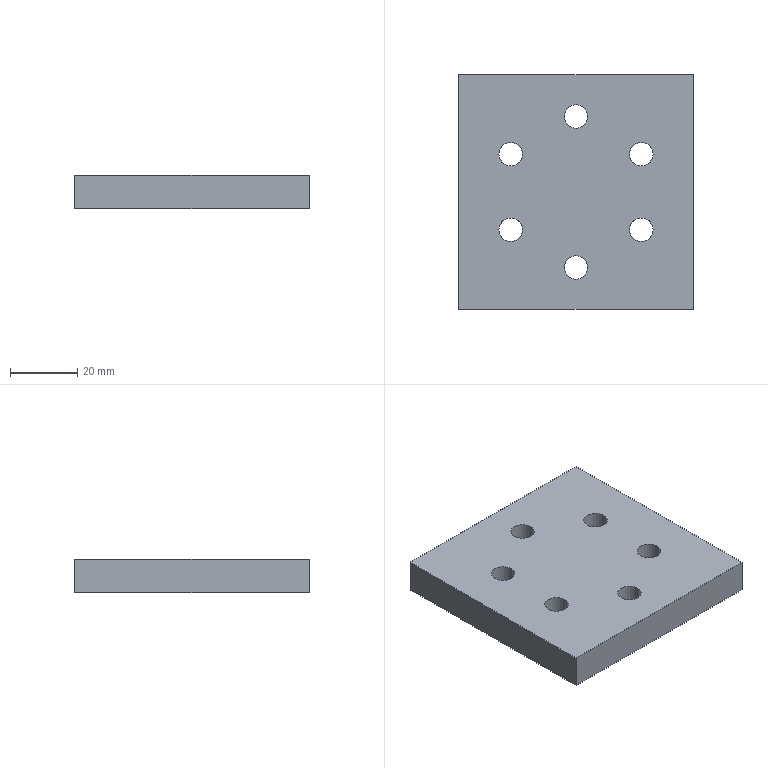Part | SolidWorks | features BaseBody 1 | 1 solid | 18 faces | box 70 x 70 x 10 mm | volume 46691 mm3 | cylinder 12 | plane 6 | commonest cylinder face diameters 7 x12
STEP:
#1=CARTESIAN_POINT('',(15.986,-11.25,0.));
#2=VERTEX_POINT('',#1);
#3=CARTESIAN_POINT('',(22.986,-11.25,0.));
#4=VERTEX_POINT('',#3);
#5=CARTESIAN_POINT('',(19.486,-11.25,0.));
#6=DIRECTION('',(0.,0.,1.));
#7=DIRECTION('',(1.,0.,0.));
#8=AXIS2_PLACEMENT_3D('',#5,#6,#7);
#9=CIRCLE('',#8,3.5);
#10=EDGE_CURVE('',#2,#4,#9,.T.);
#11=ORIENTED_EDGE('',*,*,#10,.F.);
#12=CARTESIAN_POINT('',(15.986,-11.25,10.));
#13=VERTEX_POINT('',#12);
#14=CARTESIAN_POINT('',(15.986,-11.25,10.));
#15=DIRECTION('',(0.,0.,1.));
#16=VECTOR('',#15,1000.);
#17=LINE('',#14,#16);
#18=EDGE_CURVE('',#2,#13,#17,.T.);
#19=ORIENTED_EDGE('',*,*,#18,.T.);
#20=CARTESIAN_POINT('',(22.986,-11.25,10.));
#21=VERTEX_POINT('',#20);
#22=CARTESIAN_POINT('',(19.486,-11.25,10.));
#23=DIRECTION('',(0.,0.,1.));
#24=DIRECTION('',(1.,0.,0.));
#25=AXIS2_PLACEMENT_3D('',#22,#23,#24);
#26=CIRCLE('',#25,3.5);
#27=EDGE_CURVE('',#13,#21,#26,.T.);
#28=ORIENTED_EDGE('',*,*,#27,.T.);
#29=CARTESIAN_POINT('',(22.986,-11.25,10.));
#30=DIRECTION('',(0.,0.,1.));
#31=VECTOR('',#30,1000.);
#32=LINE('',#29,#31);
#33=EDGE_CURVE('',#4,#21,#32,.T.);
#34=ORIENTED_EDGE('',*,*,#33,.F.);
#35=EDGE_LOOP('',(#11,#19,#28,#34));
#36=FACE_OUTER_BOUND('',#35,.T.);
#37=CARTESIAN_POINT('',(19.486,-11.25,10.));
#38=DIRECTION('',(0.,0.,1.));
#39=DIRECTION('',(1.,0.,0.));
#40=AXIS2_PLACEMENT_3D('',#37,#38,#39);
#41=CYLINDRICAL_SURFACE('',#40,3.5);
#42=ADVANCED_FACE('',(#36),#41,.F.);
#43=CARTESIAN_POINT('',(-3.5,-22.5,0.));
#44=VERTEX_POINT('',#43);
#45=CARTESIAN_POINT('',(3.5,-22.5,0.));
#46=VERTEX_POINT('',#45);
#47=CARTESIAN_POINT('',(0.,-22.5,0.));
#48=DIRECTION('',(0.,0.,1.));
#49=DIRECTION('',(1.,0.,0.));
#50=AXIS2_PLACEMENT_3D('',#47,#48,#49);
#51=CIRCLE('',#50,3.5);
#52=EDGE_CURVE('',#44,#46,#51,.T.);
#53=ORIENTED_EDGE('',*,*,#52,.F.);
#54=CARTESIAN_POINT('',(-3.5,-22.5,10.));
#55=VERTEX_POINT('',#54);
#56=CARTESIAN_POINT('',(-3.5,-22.5,10.));
#57=DIRECTION('',(0.,0.,1.));
#58=VECTOR('',#57,1000.);
#59=LINE('',#56,#58);
#60=EDGE_CURVE('',#44,#55,#59,.T.);
#61=ORIENTED_EDGE('',*,*,#60,.T.);
#62=CARTESIAN_POINT('',(3.5,-22.5,10.));
#63=VERTEX_POINT('',#62);
#64=CARTESIAN_POINT('',(0.,-22.5,10.));
#65=DIRECTION('',(0.,0.,1.));
#66=DIRECTION('',(1.,0.,0.));
#67=AXIS2_PLACEMENT_3D('',#64,#65,#66);
#68=CIRCLE('',#67,3.5);
#69=EDGE_CURVE('',#55,#63,#68,.T.);
#70=ORIENTED_EDGE('',*,*,#69,.T.);
#71=CARTESIAN_POINT('',(3.5,-22.5,10.));
#72=DIRECTION('',(0.,0.,1.));
#73=VECTOR('',#72,1000.);
#74=LINE('',#71,#73);
#75=EDGE_CURVE('',#46,#63,#74,.T.);
#76=ORIENTED_EDGE('',*,*,#75,.F.);
#77=EDGE_LOOP('',(#53,#61,#70,#76));
#78=FACE_OUTER_BOUND('',#77,.T.);
#79=CARTESIAN_POINT('',(0.,-22.5,10.));
#80=DIRECTION('',(0.,0.,1.));
#81=DIRECTION('',(1.,0.,0.));
#82=AXIS2_PLACEMENT_3D('',#79,#80,#81);
#83=CYLINDRICAL_SURFACE('',#82,3.5);
#84=ADVANCED_FACE('',(#78),#83,.F.);
#85=CARTESIAN_POINT('',(-22.986,-11.25,0.));
#86=VERTEX_POINT('',#85);
#87=CARTESIAN_POINT('',(-15.986,-11.25,0.));
#88=VERTEX_POINT('',#87);
#89=CARTESIAN_POINT('',(-19.486,-11.25,0.));
#90=DIRECTION('',(0.,0.,1.));
#91=DIRECTION('',(1.,0.,0.));
#92=AXIS2_PLACEMENT_3D('',#89,#90,#91);
#93=CIRCLE('',#92,3.5);
#94=EDGE_CURVE('',#86,#88,#93,.T.);
#95=ORIENTED_EDGE('',*,*,#94,.F.);
#96=CARTESIAN_POINT('',(-22.986,-11.25,10.));
#97=VERTEX_POINT('',#96);
#98=CARTESIAN_POINT('',(-22.986,-11.25,10.));
#99=DIRECTION('',(0.,0.,1.));
#100=VECTOR('',#99,1000.);
#101=LINE('',#98,#100);
#102=EDGE_CURVE('',#86,#97,#101,.T.);
#103=ORIENTED_EDGE('',*,*,#102,.T.);
#104=CARTESIAN_POINT('',(-15.986,-11.25,10.));
#105=VERTEX_POINT('',#104);
#106=CARTESIAN_POINT('',(-19.486,-11.25,10.));
#107=DIRECTION('',(0.,0.,1.));
#108=DIRECTION('',(1.,0.,0.));
#109=AXIS2_PLACEMENT_3D('',#106,#107,#108);
#110=CIRCLE('',#109,3.5);
#111=EDGE_CURVE('',#97,#105,#110,.T.);
#112=ORIENTED_EDGE('',*,*,#111,.T.);
#113=CARTESIAN_POINT('',(-15.986,-11.25,10.));
#114=DIRECTION('',(0.,0.,1.));
#115=VECTOR('',#114,1000.);
#116=LINE('',#113,#115);
#117=EDGE_CURVE('',#88,#105,#116,.T.);
#118=ORIENTED_EDGE('',*,*,#117,.F.);
#119=EDGE_LOOP('',(#95,#103,#112,#118));
#120=FACE_OUTER_BOUND('',#119,.T.);
#121=CARTESIAN_POINT('',(-19.486,-11.25,10.));
#122=DIRECTION('',(0.,0.,1.));
#123=DIRECTION('',(1.,0.,0.));
#124=AXIS2_PLACEMENT_3D('',#121,#122,#123);
#125=CYLINDRICAL_SURFACE('',#124,3.5);
#126=ADVANCED_FACE('',(#120),#125,.F.);
#127=CARTESIAN_POINT('',(-22.986,11.25,0.));
#128=VERTEX_POINT('',#127);
#129=CARTESIAN_POINT('',(-15.986,11.25,0.));
#130=VERTEX_POINT('',#129);
#131=CARTESIAN_POINT('',(-19.486,11.25,0.));
#132=DIRECTION('',(0.,0.,1.));
#133=DIRECTION('',(1.,0.,0.));
#134=AXIS2_PLACEMENT_3D('',#131,#132,#133);
#135=CIRCLE('',#134,3.5);
#136=EDGE_CURVE('',#128,#130,#135,.T.);
#137=ORIENTED_EDGE('',*,*,#136,.F.);
#138=CARTESIAN_POINT('',(-22.986,11.25,10.));
#139=VERTEX_POINT('',#138);
#140=CARTESIAN_POINT('',(-22.986,11.25,10.));
#141=DIRECTION('',(0.,0.,1.));
#142=VECTOR('',#141,1000.);
#143=LINE('',#140,#142);
#144=EDGE_CURVE('',#128,#139,#143,.T.);
#145=ORIENTED_EDGE('',*,*,#144,.T.);
#146=CARTESIAN_POINT('',(-15.986,11.25,10.));
#147=VERTEX_POINT('',#146);
#148=CARTESIAN_POINT('',(-19.486,11.25,10.));
#149=DIRECTION('',(0.,0.,1.));
#150=DIRECTION('',(1.,0.,0.));
#151=AXIS2_PLACEMENT_3D('',#148,#149,#150);
#152=CIRCLE('',#151,3.5);
#153=EDGE_CURVE('',#139,#147,#152,.T.);
#154=ORIENTED_EDGE('',*,*,#153,.T.);
#155=CARTESIAN_POINT('',(-15.986,11.25,10.));
#156=DIRECTION('',(0.,0.,1.));
#157=VECTOR('',#156,1000.);
#158=LINE('',#155,#157);
#159=EDGE_CURVE('',#130,#147,#158,.T.);
#160=ORIENTED_EDGE('',*,*,#159,.F.);
#161=EDGE_LOOP('',(#137,#145,#154,#160));
#162=FACE_OUTER_BOUND('',#161,.T.);
#163=CARTESIAN_POINT('',(-19.486,11.25,10.));
#164=DIRECTION('',(0.,0.,1.));
#165=DIRECTION('',(1.,0.,0.));
#166=AXIS2_PLACEMENT_3D('',#163,#164,#165);
#167=CYLINDRICAL_SURFACE('',#166,3.5);
#168=ADVANCED_FACE('',(#162),#167,.F.);
#169=CARTESIAN_POINT('',(-3.5,22.5,0.));
#170=VERTEX_POINT('',#169);
#171=CARTESIAN_POINT('',(3.5,22.5,0.));
#172=VERTEX_POINT('',#171);
#173=CARTESIAN_POINT('',(0.,22.5,0.));
#174=DIRECTION('',(0.,0.,1.));
#175=DIRECTION('',(1.,0.,0.));
#176=AXIS2_PLACEMENT_3D('',#173,#174,#175);
#177=CIRCLE('',#176,3.5);
#178=EDGE_CURVE('',#170,#172,#177,.T.);
#179=ORIENTED_EDGE('',*,*,#178,.F.);
#180=CARTESIAN_POINT('',(-3.5,22.5,10.));
#181=VERTEX_POINT('',#180);
#182=CARTESIAN_POINT('',(-3.5,22.5,10.));
#183=DIRECTION('',(0.,0.,1.));
#184=VECTOR('',#183,1000.);
#185=LINE('',#182,#184);
#186=EDGE_CURVE('',#170,#181,#185,.T.);
#187=ORIENTED_EDGE('',*,*,#186,.T.);
#188=CARTESIAN_POINT('',(3.5,22.5,10.));
#189=VERTEX_POINT('',#188);
#190=CARTESIAN_POINT('',(0.,22.5,10.));
#191=DIRECTION('',(0.,0.,1.));
#192=DIRECTION('',(1.,0.,0.));
#193=AXIS2_PLACEMENT_3D('',#190,#191,#192);
#194=CIRCLE('',#193,3.5);
#195=EDGE_CURVE('',#181,#189,#194,.T.);
#196=ORIENTED_EDGE('',*,*,#195,.T.);
#197=CARTESIAN_POINT('',(3.5,22.5,10.));
#198=DIRECTION('',(0.,0.,1.));
#199=VECTOR('',#198,1000.);
#200=LINE('',#197,#199);
#201=EDGE_CURVE('',#172,#189,#200,.T.);
#202=ORIENTED_EDGE('',*,*,#201,.F.);
#203=EDGE_LOOP('',(#179,#187,#196,#202));
#204=FACE_OUTER_BOUND('',#203,.T.);
#205=CARTESIAN_POINT('',(0.,22.5,10.));
#206=DIRECTION('',(0.,0.,1.));
#207=DIRECTION('',(1.,0.,0.));
#208=AXIS2_PLACEMENT_3D('',#205,#206,#207);
#209=CYLINDRICAL_SURFACE('',#208,3.5);
#210=ADVANCED_FACE('',(#204),#209,.F.);
#211=CARTESIAN_POINT('',(15.986,11.25,0.));
#212=VERTEX_POINT('',#211);
#213=CARTESIAN_POINT('',(22.986,11.25,0.));
#214=VERTEX_POINT('',#213);
#215=CARTESIAN_POINT('',(19.486,11.25,0.));
#216=DIRECTION('',(0.,0.,1.));
#217=DIRECTION('',(1.,0.,0.));
#218=AXIS2_PLACEMENT_3D('',#215,#216,#217);
#219=CIRCLE('',#218,3.5);
#220=EDGE_CURVE('',#212,#214,#219,.T.);
#221=ORIENTED_EDGE('',*,*,#220,.F.);
#222=CARTESIAN_POINT('',(15.986,11.25,10.));
#223=VERTEX_POINT('',#222);
#224=CARTESIAN_POINT('',(15.986,11.25,10.));
#225=DIRECTION('',(0.,0.,1.));
#226=VECTOR('',#225,1000.);
#227=LINE('',#224,#226);
#228=EDGE_CURVE('',#212,#223,#227,.T.);
#229=ORIENTED_EDGE('',*,*,#228,.T.);
#230=CARTESIAN_POINT('',(22.986,11.25,10.));
#231=VERTEX_POINT('',#230);
#232=CARTESIAN_POINT('',(19.486,11.25,10.));
#233=DIRECTION('',(0.,0.,1.));
#234=DIRECTION('',(1.,0.,0.));
#235=AXIS2_PLACEMENT_3D('',#232,#233,#234);
#236=CIRCLE('',#235,3.5);
#237=EDGE_CURVE('',#223,#231,#236,.T.);
#238=ORIENTED_EDGE('',*,*,#237,.T.);
#239=CARTESIAN_POINT('',(22.986,11.25,10.));
#240=DIRECTION('',(0.,0.,1.));
#241=VECTOR('',#240,1000.);
#242=LINE('',#239,#241);
#243=EDGE_CURVE('',#214,#231,#242,.T.);
#244=ORIENTED_EDGE('',*,*,#243,.F.);
#245=EDGE_LOOP('',(#221,#229,#238,#244));
#246=FACE_OUTER_BOUND('',#245,.T.);
#247=CARTESIAN_POINT('',(19.486,11.25,10.));
#248=DIRECTION('',(0.,0.,1.));
#249=DIRECTION('',(1.,0.,0.));
#250=AXIS2_PLACEMENT_3D('',#247,#248,#249);
#251=CYLINDRICAL_SURFACE('',#250,3.5);
#252=ADVANCED_FACE('',(#246),#251,.F.);
#253=CARTESIAN_POINT('',(35.,-35.,0.));
#254=VERTEX_POINT('',#253);
#255=CARTESIAN_POINT('',(35.,35.,0.));
#256=VERTEX_POINT('',#255);
#257=CARTESIAN_POINT('',(35.,35.,0.));
#258=DIRECTION('',(0.,1.,0.));
#259=VECTOR('',#258,1000.);
#260=LINE('',#257,#259);
#261=EDGE_CURVE('',#254,#256,#260,.T.);
#262=ORIENTED_EDGE('',*,*,#261,.T.);
#263=CARTESIAN_POINT('',(35.,35.,10.));
#264=VERTEX_POINT('',#263);
#265=CARTESIAN_POINT('',(35.,35.,10.));
#266=DIRECTION('',(0.,0.,-1.));
#267=VECTOR('',#266,1000.);
#268=LINE('',#265,#267);
#269=EDGE_CURVE('',#264,#256,#268,.T.);
#270=ORIENTED_EDGE('',*,*,#269,.F.);
#271=CARTESIAN_POINT('',(35.,-35.,10.));
#272=VERTEX_POINT('',#271);
#273=CARTESIAN_POINT('',(35.,35.,10.));
#274=DIRECTION('',(0.,1.,0.));
#275=VECTOR('',#274,1000.);
#276=LINE('',#273,#275);
#277=EDGE_CURVE('',#272,#264,#276,.T.);
#278=ORIENTED_EDGE('',*,*,#277,.F.);
#279=CARTESIAN_POINT('',(35.,-35.,10.));
#280=DIRECTION('',(0.,0.,-1.));
#281=VECTOR('',#280,1000.);
#282=LINE('',#279,#281);
#283=EDGE_CURVE('',#272,#254,#282,.T.);
#284=ORIENTED_EDGE('',*,*,#283,.T.);
#285=EDGE_LOOP('',(#262,#270,#278,#284));
#286=FACE_OUTER_BOUND('',#285,.T.);
#287=CARTESIAN_POINT('',(35.,35.,10.));
#288=DIRECTION('',(-1.,0.,0.));
#289=DIRECTION('',(0.,-1.,0.));
#290=AXIS2_PLACEMENT_3D('',#287,#288,#289);
#291=PLANE('',#290);
#292=ADVANCED_FACE('',(#286),#291,.F.);
#293=CARTESIAN_POINT('',(-35.,35.,0.));
#294=VERTEX_POINT('',#293);
#295=CARTESIAN_POINT('',(-35.,35.,0.));
#296=DIRECTION('',(-1.,0.,0.));
#297=VECTOR('',#296,1000.);
#298=LINE('',#295,#297);
#299=EDGE_CURVE('',#256,#294,#298,.T.);
#300=ORIENTED_EDGE('',*,*,#299,.T.);
#301=CARTESIAN_POINT('',(-35.,35.,10.));
#302=VERTEX_POINT('',#301);
#303=CARTESIAN_POINT('',(-35.,35.,10.));
#304=DIRECTION('',(0.,0.,-1.));
#305=VECTOR('',#304,1000.);
#306=LINE('',#303,#305);
#307=EDGE_CURVE('',#302,#294,#306,.T.);
#308=ORIENTED_EDGE('',*,*,#307,.F.);
#309=CARTESIAN_POINT('',(-35.,35.,10.));
#310=DIRECTION('',(-1.,0.,0.));
#311=VECTOR('',#310,1000.);
#312=LINE('',#309,#311);
#313=EDGE_CURVE('',#264,#302,#312,.T.);
#314=ORIENTED_EDGE('',*,*,#313,.F.);
#315=ORIENTED_EDGE('',*,*,#269,.T.);
#316=EDGE_LOOP('',(#300,#308,#314,#315));
#317=FACE_OUTER_BOUND('',#316,.T.);
#318=CARTESIAN_POINT('',(-35.,35.,10.));
#319=DIRECTION('',(0.,-1.,0.));
#320=DIRECTION('',(0.,0.,-1.));
#321=AXIS2_PLACEMENT_3D('',#318,#319,#320);
#322=PLANE('',#321);
#323=ADVANCED_FACE('',(#317),#322,.F.);
#324=CARTESIAN_POINT('',(-35.,-35.,0.));
#325=VERTEX_POINT('',#324);
#326=CARTESIAN_POINT('',(-35.,35.,0.));
#327=DIRECTION('',(0.,-1.,0.));
#328=VECTOR('',#327,1000.);
#329=LINE('',#326,#328);
#330=EDGE_CURVE('',#294,#325,#329,.T.);
#331=ORIENTED_EDGE('',*,*,#330,.T.);
#332=CARTESIAN_POINT('',(-35.,-35.,10.));
#333=VERTEX_POINT('',#332);
#334=CARTESIAN_POINT('',(-35.,-35.,10.));
#335=DIRECTION('',(0.,0.,-1.));
#336=VECTOR('',#335,1000.);
#337=LINE('',#334,#336);
#338=EDGE_CURVE('',#333,#325,#337,.T.);
#339=ORIENTED_EDGE('',*,*,#338,.F.);
#340=CARTESIAN_POINT('',(-35.,35.,10.));
#341=DIRECTION('',(0.,-1.,0.));
#342=VECTOR('',#341,1000.);
#343=LINE('',#340,#342);
#344=EDGE_CURVE('',#302,#333,#343,.T.);
#345=ORIENTED_EDGE('',*,*,#344,.F.);
#346=ORIENTED_EDGE('',*,*,#307,.T.);
#347=EDGE_LOOP('',(#331,#339,#345,#346));
#348=FACE_OUTER_BOUND('',#347,.T.);
#349=CARTESIAN_POINT('',(-35.,35.,10.));
#350=DIRECTION('',(1.,0.,0.));
#351=DIRECTION('',(0.,1.,0.));
#352=AXIS2_PLACEMENT_3D('',#349,#350,#351);
#353=PLANE('',#352);
#354=ADVANCED_FACE('',(#348),#353,.F.);
#355=CARTESIAN_POINT('',(-35.,-35.,0.));
#356=DIRECTION('',(1.,0.,0.));
#357=VECTOR('',#356,1000.);
#358=LINE('',#355,#357);
#359=EDGE_CURVE('',#325,#254,#358,.T.);
#360=ORIENTED_EDGE('',*,*,#359,.T.);
#361=ORIENTED_EDGE('',*,*,#283,.F.);
#362=CARTESIAN_POINT('',(-35.,-35.,10.));
#363=DIRECTION('',(1.,0.,0.));
#364=VECTOR('',#363,1000.);
#365=LINE('',#362,#364);
#366=EDGE_CURVE('',#333,#272,#365,.T.);
#367=ORIENTED_EDGE('',*,*,#366,.F.);
#368=ORIENTED_EDGE('',*,*,#338,.T.);
#369=EDGE_LOOP('',(#360,#361,#367,#368));
#370=FACE_OUTER_BOUND('',#369,.T.);
#371=CARTESIAN_POINT('',(-35.,-35.,10.));
#372=DIRECTION('',(0.,1.,0.));
#373=DIRECTION('',(0.,0.,1.));
#374=AXIS2_PLACEMENT_3D('',#371,#372,#373);
#375=PLANE('',#374);
#376=ADVANCED_FACE('',(#370),#375,.F.);
#377=CARTESIAN_POINT('',(19.486,-11.25,10.));
#378=DIRECTION('',(0.,0.,1.));
#379=DIRECTION('',(1.,0.,0.));
#380=AXIS2_PLACEMENT_3D('',#377,#378,#379);
#381=CIRCLE('',#380,3.5);
#382=EDGE_CURVE('',#21,#13,#381,.T.);
#383=ORIENTED_EDGE('',*,*,#382,.F.);
#384=ORIENTED_EDGE('',*,*,#27,.F.);
#385=EDGE_LOOP('',(#383,#384));
#386=FACE_BOUND('',#385,.T.);
#387=CARTESIAN_POINT('',(0.,-22.5,10.));
#388=DIRECTION('',(0.,0.,1.));
#389=DIRECTION('',(1.,0.,0.));
#390=AXIS2_PLACEMENT_3D('',#387,#388,#389);
#391=CIRCLE('',#390,3.5);
#392=EDGE_CURVE('',#63,#55,#391,.T.);
#393=ORIENTED_EDGE('',*,*,#392,.F.);
#394=ORIENTED_EDGE('',*,*,#69,.F.);
#395=EDGE_LOOP('',(#393,#394));
#396=FACE_BOUND('',#395,.T.);
#397=CARTESIAN_POINT('',(-19.486,-11.25,10.));
#398=DIRECTION('',(0.,0.,1.));
#399=DIRECTION('',(1.,0.,0.));
#400=AXIS2_PLACEMENT_3D('',#397,#398,#399);
#401=CIRCLE('',#400,3.5);
#402=EDGE_CURVE('',#105,#97,#401,.T.);
#403=ORIENTED_EDGE('',*,*,#402,.F.);
#404=ORIENTED_EDGE('',*,*,#111,.F.);
#405=EDGE_LOOP('',(#403,#404));
#406=FACE_BOUND('',#405,.T.);
#407=CARTESIAN_POINT('',(-19.486,11.25,10.));
#408=DIRECTION('',(0.,0.,1.));
#409=DIRECTION('',(1.,0.,0.));
#410=AXIS2_PLACEMENT_3D('',#407,#408,#409);
#411=CIRCLE('',#410,3.5);
#412=EDGE_CURVE('',#147,#139,#411,.T.);
#413=ORIENTED_EDGE('',*,*,#412,.F.);
#414=ORIENTED_EDGE('',*,*,#153,.F.);
#415=EDGE_LOOP('',(#413,#414));
#416=FACE_BOUND('',#415,.T.);
#417=CARTESIAN_POINT('',(0.,22.5,10.));
#418=DIRECTION('',(0.,0.,1.));
#419=DIRECTION('',(1.,0.,0.));
#420=AXIS2_PLACEMENT_3D('',#417,#418,#419);
#421=CIRCLE('',#420,3.5);
#422=EDGE_CURVE('',#189,#181,#421,.T.);
#423=ORIENTED_EDGE('',*,*,#422,.F.);
#424=ORIENTED_EDGE('',*,*,#195,.F.);
#425=EDGE_LOOP('',(#423,#424));
#426=FACE_BOUND('',#425,.T.);
#427=CARTESIAN_POINT('',(19.486,11.25,10.));
#428=DIRECTION('',(0.,0.,1.));
#429=DIRECTION('',(1.,0.,0.));
#430=AXIS2_PLACEMENT_3D('',#427,#428,#429);
#431=CIRCLE('',#430,3.5);
#432=EDGE_CURVE('',#231,#223,#431,.T.);
#433=ORIENTED_EDGE('',*,*,#432,.F.);
#434=ORIENTED_EDGE('',*,*,#237,.F.);
#435=EDGE_LOOP('',(#433,#434));
#436=FACE_BOUND('',#435,.T.);
#437=ORIENTED_EDGE('',*,*,#277,.T.);
#438=ORIENTED_EDGE('',*,*,#313,.T.);
#439=ORIENTED_EDGE('',*,*,#344,.T.);
#440=ORIENTED_EDGE('',*,*,#366,.T.);
#441=EDGE_LOOP('',(#437,#438,#439,#440));
#442=FACE_OUTER_BOUND('',#441,.T.);
#443=CARTESIAN_POINT('',(0.,0.,10.));
#444=DIRECTION('',(0.,0.,1.));
#445=DIRECTION('',(1.,0.,0.));
#446=AXIS2_PLACEMENT_3D('',#443,#444,#445);
#447=PLANE('',#446);
#448=ADVANCED_FACE('',(#386,#396,#406,#416,#426,#436,#442),#447,.T.);
#449=CARTESIAN_POINT('',(19.486,-11.25,0.));
#450=DIRECTION('',(0.,0.,1.));
#451=DIRECTION('',(1.,0.,0.));
#452=AXIS2_PLACEMENT_3D('',#449,#450,#451);
#453=CIRCLE('',#452,3.5);
#454=EDGE_CURVE('',#4,#2,#453,.T.);
#455=ORIENTED_EDGE('',*,*,#454,.T.);
#456=ORIENTED_EDGE('',*,*,#10,.T.);
#457=EDGE_LOOP('',(#455,#456));
#458=FACE_BOUND('',#457,.T.);
#459=CARTESIAN_POINT('',(0.,-22.5,0.));
#460=DIRECTION('',(0.,0.,1.));
#461=DIRECTION('',(1.,0.,0.));
#462=AXIS2_PLACEMENT_3D('',#459,#460,#461);
#463=CIRCLE('',#462,3.5);
#464=EDGE_CURVE('',#46,#44,#463,.T.);
#465=ORIENTED_EDGE('',*,*,#464,.T.);
#466=ORIENTED_EDGE('',*,*,#52,.T.);
#467=EDGE_LOOP('',(#465,#466));
#468=FACE_BOUND('',#467,.T.);
#469=CARTESIAN_POINT('',(-19.486,-11.25,0.));
#470=DIRECTION('',(0.,0.,1.));
#471=DIRECTION('',(1.,0.,0.));
#472=AXIS2_PLACEMENT_3D('',#469,#470,#471);
#473=CIRCLE('',#472,3.5);
#474=EDGE_CURVE('',#88,#86,#473,.T.);
#475=ORIENTED_EDGE('',*,*,#474,.T.);
#476=ORIENTED_EDGE('',*,*,#94,.T.);
#477=EDGE_LOOP('',(#475,#476));
#478=FACE_BOUND('',#477,.T.);
#479=CARTESIAN_POINT('',(-19.486,11.25,0.));
#480=DIRECTION('',(0.,0.,1.));
#481=DIRECTION('',(1.,0.,0.));
#482=AXIS2_PLACEMENT_3D('',#479,#480,#481);
#483=CIRCLE('',#482,3.5);
#484=EDGE_CURVE('',#130,#128,#483,.T.);
#485=ORIENTED_EDGE('',*,*,#484,.T.);
#486=ORIENTED_EDGE('',*,*,#136,.T.);
#487=EDGE_LOOP('',(#485,#486));
#488=FACE_BOUND('',#487,.T.);
#489=CARTESIAN_POINT('',(0.,22.5,0.));
#490=DIRECTION('',(0.,0.,1.));
#491=DIRECTION('',(1.,0.,0.));
#492=AXIS2_PLACEMENT_3D('',#489,#490,#491);
#493=CIRCLE('',#492,3.5);
#494=EDGE_CURVE('',#172,#170,#493,.T.);
#495=ORIENTED_EDGE('',*,*,#494,.T.);
#496=ORIENTED_EDGE('',*,*,#178,.T.);
#497=EDGE_LOOP('',(#495,#496));
#498=FACE_BOUND('',#497,.T.);
#499=CARTESIAN_POINT('',(19.486,11.25,0.));
#500=DIRECTION('',(0.,0.,1.));
#501=DIRECTION('',(1.,0.,0.));
#502=AXIS2_PLACEMENT_3D('',#499,#500,#501);
#503=CIRCLE('',#502,3.5);
#504=EDGE_CURVE('',#214,#212,#503,.T.);
#505=ORIENTED_EDGE('',*,*,#504,.T.);
#506=ORIENTED_EDGE('',*,*,#220,.T.);
#507=EDGE_LOOP('',(#505,#506));
#508=FACE_BOUND('',#507,.T.);
#509=ORIENTED_EDGE('',*,*,#261,.F.);
#510=ORIENTED_EDGE('',*,*,#359,.F.);
#511=ORIENTED_EDGE('',*,*,#330,.F.);
#512=ORIENTED_EDGE('',*,*,#299,.F.);
#513=EDGE_LOOP('',(#509,#510,#511,#512));
#514=FACE_OUTER_BOUND('',#513,.T.);
#515=CARTESIAN_POINT('',(0.,0.,0.));
#516=DIRECTION('',(0.,0.,1.));
#517=DIRECTION('',(1.,0.,0.));
#518=AXIS2_PLACEMENT_3D('',#515,#516,#517);
#519=PLANE('',#518);
#520=ADVANCED_FACE('',(#458,#468,#478,#488,#498,#508,#514),#519,.F.);
#521=ORIENTED_EDGE('',*,*,#228,.F.);
#522=ORIENTED_EDGE('',*,*,#504,.F.);
#523=ORIENTED_EDGE('',*,*,#243,.T.);
#524=ORIENTED_EDGE('',*,*,#432,.T.);
#525=EDGE_LOOP('',(#521,#522,#523,#524));
#526=FACE_OUTER_BOUND('',#525,.T.);
#527=CARTESIAN_POINT('',(19.486,11.25,10.));
#528=DIRECTION('',(0.,0.,1.));
#529=DIRECTION('',(1.,0.,0.));
#530=AXIS2_PLACEMENT_3D('',#527,#528,#529);
#531=CYLINDRICAL_SURFACE('',#530,3.5);
#532=ADVANCED_FACE('',(#526),#531,.F.);
#533=ORIENTED_EDGE('',*,*,#186,.F.);
#534=ORIENTED_EDGE('',*,*,#494,.F.);
#535=ORIENTED_EDGE('',*,*,#201,.T.);
#536=ORIENTED_EDGE('',*,*,#422,.T.);
#537=EDGE_LOOP('',(#533,#534,#535,#536));
#538=FACE_OUTER_BOUND('',#537,.T.);
#539=CARTESIAN_POINT('',(0.,22.5,10.));
#540=DIRECTION('',(0.,0.,1.));
#541=DIRECTION('',(1.,0.,0.));
#542=AXIS2_PLACEMENT_3D('',#539,#540,#541);
#543=CYLINDRICAL_SURFACE('',#542,3.5);
#544=ADVANCED_FACE('',(#538),#543,.F.);
#545=ORIENTED_EDGE('',*,*,#144,.F.);
#546=ORIENTED_EDGE('',*,*,#484,.F.);
#547=ORIENTED_EDGE('',*,*,#159,.T.);
#548=ORIENTED_EDGE('',*,*,#412,.T.);
#549=EDGE_LOOP('',(#545,#546,#547,#548));
#550=FACE_OUTER_BOUND('',#549,.T.);
#551=CARTESIAN_POINT('',(-19.486,11.25,10.));
#552=DIRECTION('',(0.,0.,1.));
#553=DIRECTION('',(1.,0.,0.));
#554=AXIS2_PLACEMENT_3D('',#551,#552,#553);
#555=CYLINDRICAL_SURFACE('',#554,3.5);
#556=ADVANCED_FACE('',(#550),#555,.F.);
#557=ORIENTED_EDGE('',*,*,#102,.F.);
#558=ORIENTED_EDGE('',*,*,#474,.F.);
#559=ORIENTED_EDGE('',*,*,#117,.T.);
#560=ORIENTED_EDGE('',*,*,#402,.T.);
#561=EDGE_LOOP('',(#557,#558,#559,#560));
#562=FACE_OUTER_BOUND('',#561,.T.);
#563=CARTESIAN_POINT('',(-19.486,-11.25,10.));
#564=DIRECTION('',(0.,0.,1.));
#565=DIRECTION('',(1.,0.,0.));
#566=AXIS2_PLACEMENT_3D('',#563,#564,#565);
#567=CYLINDRICAL_SURFACE('',#566,3.5);
#568=ADVANCED_FACE('',(#562),#567,.F.);
#569=ORIENTED_EDGE('',*,*,#60,.F.);
#570=ORIENTED_EDGE('',*,*,#464,.F.);
#571=ORIENTED_EDGE('',*,*,#75,.T.);
#572=ORIENTED_EDGE('',*,*,#392,.T.);
#573=EDGE_LOOP('',(#569,#570,#571,#572));
#574=FACE_OUTER_BOUND('',#573,.T.);
#575=CARTESIAN_POINT('',(0.,-22.5,10.));
#576=DIRECTION('',(0.,0.,1.));
#577=DIRECTION('',(1.,0.,0.));
#578=AXIS2_PLACEMENT_3D('',#575,#576,#577);
#579=CYLINDRICAL_SURFACE('',#578,3.5);
#580=ADVANCED_FACE('',(#574),#579,.F.);
#581=ORIENTED_EDGE('',*,*,#18,.F.);
#582=ORIENTED_EDGE('',*,*,#454,.F.);
#583=ORIENTED_EDGE('',*,*,#33,.T.);
#584=ORIENTED_EDGE('',*,*,#382,.T.);
#585=EDGE_LOOP('',(#581,#582,#583,#584));
#586=FACE_OUTER_BOUND('',#585,.T.);
#587=CARTESIAN_POINT('',(19.486,-11.25,10.));
#588=DIRECTION('',(0.,0.,1.));
#589=DIRECTION('',(1.,0.,0.));
#590=AXIS2_PLACEMENT_3D('',#587,#588,#589);
#591=CYLINDRICAL_SURFACE('',#590,3.5);
#592=ADVANCED_FACE('',(#586),#591,.F.);
#593=CLOSED_SHELL('',(#42,#84,#126,#168,#210,#252,#292,#323,#354,#376,#448,#520,#532,#544,#556,#568,#580,#592));
#594=MANIFOLD_SOLID_BREP('',#593);
#595=CARTESIAN_POINT('',(0.,0.,0.));
#596=DIRECTION('',(0.,0.,1.));
#597=DIRECTION('',(1.,0.,0.));
#598=AXIS2_PLACEMENT_3D('',#595,#596,#597);
#599=(LENGTH_UNIT()NAMED_UNIT(*)SI_UNIT(.MILLI.,.METRE.));
#600=UNCERTAINTY_MEASURE_WITH_UNIT(LENGTH_MEASURE(0.00001),#599,'','');
#601=(NAMED_UNIT(*)PLANE_ANGLE_UNIT()SI_UNIT($,.RADIAN.));
#602=(NAMED_UNIT(*)SI_UNIT($,.STERADIAN.)SOLID_ANGLE_UNIT());
#603=(GEOMETRIC_REPRESENTATION_CONTEXT(3)GLOBAL_UNCERTAINTY_ASSIGNED_CONTEXT((#600))GLOBAL_UNIT_ASSIGNED_CONTEXT((#599,#601,#602))REPRESENTATION_CONTEXT('',''));
#604=ADVANCED_BREP_SHAPE_REPRESENTATION('',(#594,#598),#603);